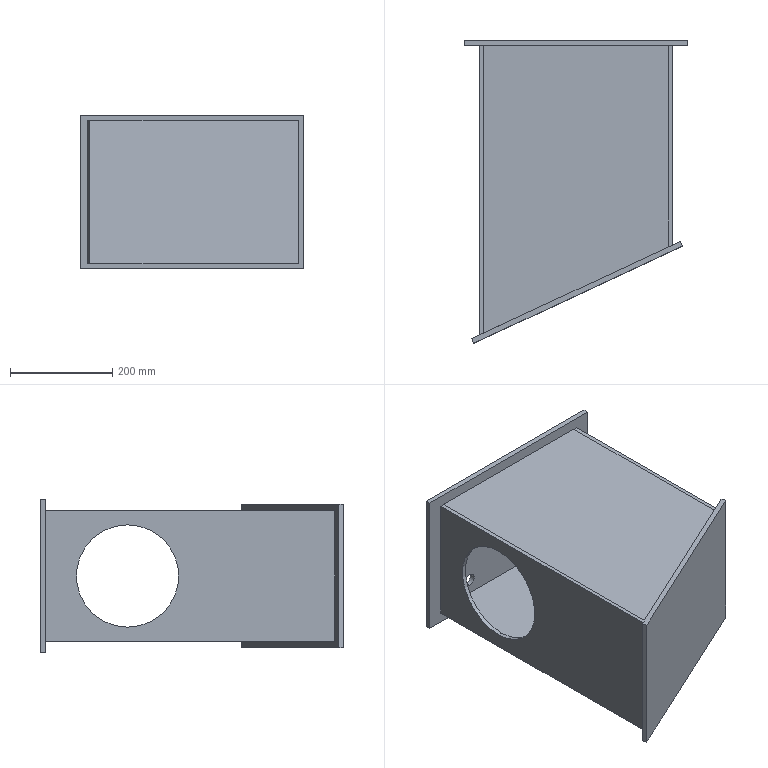Part | STEP file | Motor lower seat 1_Default<As machined> | 6 solids | 48 faces | box 436 x 591.846 x 300 mm | volume 6753859 mm3 | plane 36 | cylinder 12 | commonest cylinder face diameters 25 x8 200 x4